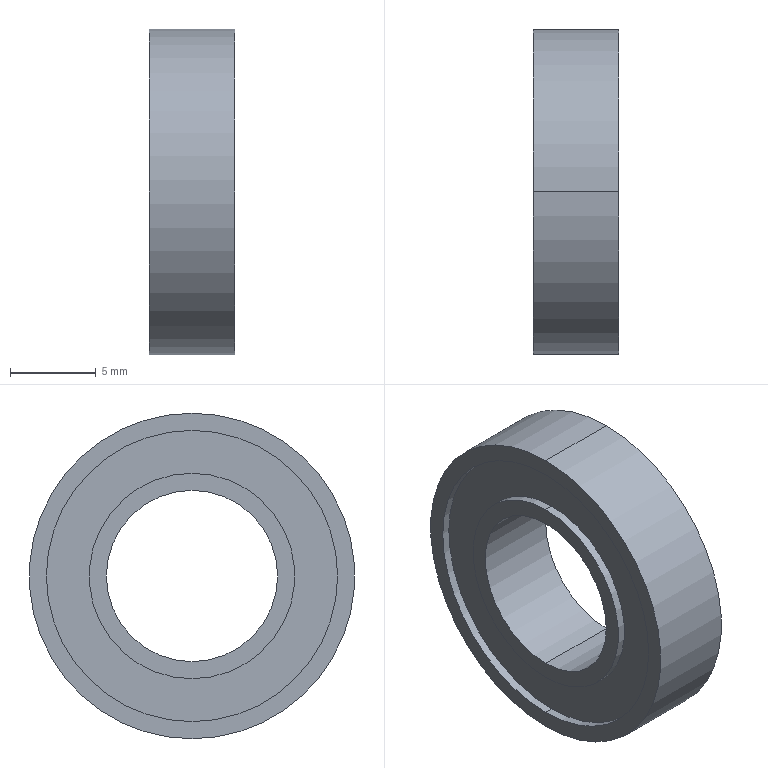Part | STEP file | Guide wheel mechanism revised.sldasm-Part-353 | 1 solid | 18 faces | box 5 x 19 x 19 mm | volume 911.062 mm3 | cylinder 12 | plane 6 | commonest cylinder face diameters 12 x4 17 x4 10 x2 19 x2
STEP:
#1=CARTESIAN_POINT('',(5.,0.,6.));
#2=VERTEX_POINT('',#1);
#3=CARTESIAN_POINT('',(5.,0.,-6.));
#4=VERTEX_POINT('',#3);
#5=CARTESIAN_POINT('',(5.,0.,0.));
#6=DIRECTION('',(-1.,0.,0.));
#7=DIRECTION('',(0.,0.,1.));
#8=AXIS2_PLACEMENT_3D('',#5,#6,#7);
#9=CIRCLE('',#8,6.);
#10=EDGE_CURVE('',#2,#4,#9,.T.);
#11=ORIENTED_EDGE('',*,*,#10,.T.);
#12=CARTESIAN_POINT('',(4.5,0.,-6.));
#13=VERTEX_POINT('',#12);
#14=CARTESIAN_POINT('',(0.,0.,-6.));
#15=DIRECTION('',(-1.,0.,0.));
#16=VECTOR('',#15,1000.);
#17=LINE('',#14,#16);
#18=EDGE_CURVE('',#4,#13,#17,.T.);
#19=ORIENTED_EDGE('',*,*,#18,.T.);
#20=CARTESIAN_POINT('',(4.5,0.,6.));
#21=VERTEX_POINT('',#20);
#22=CARTESIAN_POINT('',(4.5,0.,0.));
#23=DIRECTION('',(-1.,0.,0.));
#24=DIRECTION('',(0.,0.,1.));
#25=AXIS2_PLACEMENT_3D('',#22,#23,#24);
#26=CIRCLE('',#25,6.);
#27=EDGE_CURVE('',#21,#13,#26,.T.);
#28=ORIENTED_EDGE('',*,*,#27,.F.);
#29=CARTESIAN_POINT('',(0.,0.,6.));
#30=DIRECTION('',(-1.,0.,0.));
#31=VECTOR('',#30,1000.);
#32=LINE('',#29,#31);
#33=EDGE_CURVE('',#2,#21,#32,.T.);
#34=ORIENTED_EDGE('',*,*,#33,.F.);
#35=EDGE_LOOP('',(#11,#19,#28,#34));
#36=FACE_OUTER_BOUND('',#35,.T.);
#37=CARTESIAN_POINT('',(0.,0.,0.));
#38=DIRECTION('',(-1.,0.,0.));
#39=DIRECTION('',(0.,0.,1.));
#40=AXIS2_PLACEMENT_3D('',#37,#38,#39);
#41=CYLINDRICAL_SURFACE('',#40,6.);
#42=ADVANCED_FACE('',(#36),#41,.T.);
#43=CARTESIAN_POINT('',(5.,0.,-8.5));
#44=VERTEX_POINT('',#43);
#45=CARTESIAN_POINT('',(5.,0.,8.5));
#46=VERTEX_POINT('',#45);
#47=CARTESIAN_POINT('',(5.,0.,0.));
#48=DIRECTION('',(-1.,0.,0.));
#49=DIRECTION('',(0.,0.,1.));
#50=AXIS2_PLACEMENT_3D('',#47,#48,#49);
#51=CIRCLE('',#50,8.5);
#52=EDGE_CURVE('',#44,#46,#51,.T.);
#53=ORIENTED_EDGE('',*,*,#52,.F.);
#54=CARTESIAN_POINT('',(4.5,0.,-8.5));
#55=VERTEX_POINT('',#54);
#56=CARTESIAN_POINT('',(0.,0.,-8.5));
#57=DIRECTION('',(-1.,0.,0.));
#58=VECTOR('',#57,1000.);
#59=LINE('',#56,#58);
#60=EDGE_CURVE('',#44,#55,#59,.T.);
#61=ORIENTED_EDGE('',*,*,#60,.T.);
#62=CARTESIAN_POINT('',(4.5,0.,8.5));
#63=VERTEX_POINT('',#62);
#64=CARTESIAN_POINT('',(4.5,0.,0.));
#65=DIRECTION('',(-1.,0.,0.));
#66=DIRECTION('',(0.,0.,1.));
#67=AXIS2_PLACEMENT_3D('',#64,#65,#66);
#68=CIRCLE('',#67,8.5);
#69=EDGE_CURVE('',#55,#63,#68,.T.);
#70=ORIENTED_EDGE('',*,*,#69,.T.);
#71=CARTESIAN_POINT('',(0.,0.,8.5));
#72=DIRECTION('',(-1.,0.,0.));
#73=VECTOR('',#72,1000.);
#74=LINE('',#71,#73);
#75=EDGE_CURVE('',#46,#63,#74,.T.);
#76=ORIENTED_EDGE('',*,*,#75,.F.);
#77=EDGE_LOOP('',(#53,#61,#70,#76));
#78=FACE_OUTER_BOUND('',#77,.T.);
#79=CARTESIAN_POINT('',(0.,0.,0.));
#80=DIRECTION('',(-1.,0.,0.));
#81=DIRECTION('',(0.,0.,1.));
#82=AXIS2_PLACEMENT_3D('',#79,#80,#81);
#83=CYLINDRICAL_SURFACE('',#82,8.5);
#84=ADVANCED_FACE('',(#78),#83,.F.);
#85=CARTESIAN_POINT('',(5.,0.,9.5));
#86=VERTEX_POINT('',#85);
#87=CARTESIAN_POINT('',(5.,0.,-9.5));
#88=VERTEX_POINT('',#87);
#89=CARTESIAN_POINT('',(5.,0.,0.));
#90=DIRECTION('',(-1.,0.,0.));
#91=DIRECTION('',(0.,0.,1.));
#92=AXIS2_PLACEMENT_3D('',#89,#90,#91);
#93=CIRCLE('',#92,9.5);
#94=EDGE_CURVE('',#86,#88,#93,.T.);
#95=ORIENTED_EDGE('',*,*,#94,.T.);
#96=CARTESIAN_POINT('',(0.,0.,-9.5));
#97=VERTEX_POINT('',#96);
#98=CARTESIAN_POINT('',(0.,0.,-9.5));
#99=DIRECTION('',(-1.,0.,0.));
#100=VECTOR('',#99,1000.);
#101=LINE('',#98,#100);
#102=EDGE_CURVE('',#88,#97,#101,.T.);
#103=ORIENTED_EDGE('',*,*,#102,.T.);
#104=CARTESIAN_POINT('',(0.,0.,9.5));
#105=VERTEX_POINT('',#104);
#106=CARTESIAN_POINT('',(0.,0.,0.));
#107=DIRECTION('',(-1.,0.,0.));
#108=DIRECTION('',(0.,0.,1.));
#109=AXIS2_PLACEMENT_3D('',#106,#107,#108);
#110=CIRCLE('',#109,9.5);
#111=EDGE_CURVE('',#105,#97,#110,.T.);
#112=ORIENTED_EDGE('',*,*,#111,.F.);
#113=CARTESIAN_POINT('',(0.,0.,9.5));
#114=DIRECTION('',(-1.,0.,0.));
#115=VECTOR('',#114,1000.);
#116=LINE('',#113,#115);
#117=EDGE_CURVE('',#86,#105,#116,.T.);
#118=ORIENTED_EDGE('',*,*,#117,.F.);
#119=EDGE_LOOP('',(#95,#103,#112,#118));
#120=FACE_OUTER_BOUND('',#119,.T.);
#121=CARTESIAN_POINT('',(0.,0.,0.));
#122=DIRECTION('',(-1.,0.,0.));
#123=DIRECTION('',(0.,0.,1.));
#124=AXIS2_PLACEMENT_3D('',#121,#122,#123);
#125=CYLINDRICAL_SURFACE('',#124,9.5);
#126=ADVANCED_FACE('',(#120),#125,.T.);
#127=CARTESIAN_POINT('',(0.5,0.,-8.5));
#128=VERTEX_POINT('',#127);
#129=CARTESIAN_POINT('',(0.5,0.,8.5));
#130=VERTEX_POINT('',#129);
#131=CARTESIAN_POINT('',(0.5,0.,0.));
#132=DIRECTION('',(-1.,0.,0.));
#133=DIRECTION('',(0.,0.,1.));
#134=AXIS2_PLACEMENT_3D('',#131,#132,#133);
#135=CIRCLE('',#134,8.5);
#136=EDGE_CURVE('',#128,#130,#135,.T.);
#137=ORIENTED_EDGE('',*,*,#136,.F.);
#138=CARTESIAN_POINT('',(0.,0.,-8.5));
#139=VERTEX_POINT('',#138);
#140=CARTESIAN_POINT('',(0.,0.,-8.5));
#141=DIRECTION('',(-1.,0.,0.));
#142=VECTOR('',#141,1000.);
#143=LINE('',#140,#142);
#144=EDGE_CURVE('',#128,#139,#143,.T.);
#145=ORIENTED_EDGE('',*,*,#144,.T.);
#146=CARTESIAN_POINT('',(0.,0.,8.5));
#147=VERTEX_POINT('',#146);
#148=CARTESIAN_POINT('',(0.,0.,0.));
#149=DIRECTION('',(-1.,0.,0.));
#150=DIRECTION('',(0.,0.,1.));
#151=AXIS2_PLACEMENT_3D('',#148,#149,#150);
#152=CIRCLE('',#151,8.5);
#153=EDGE_CURVE('',#139,#147,#152,.T.);
#154=ORIENTED_EDGE('',*,*,#153,.T.);
#155=CARTESIAN_POINT('',(0.,0.,8.5));
#156=DIRECTION('',(-1.,0.,0.));
#157=VECTOR('',#156,1000.);
#158=LINE('',#155,#157);
#159=EDGE_CURVE('',#130,#147,#158,.T.);
#160=ORIENTED_EDGE('',*,*,#159,.F.);
#161=EDGE_LOOP('',(#137,#145,#154,#160));
#162=FACE_OUTER_BOUND('',#161,.T.);
#163=CARTESIAN_POINT('',(0.,0.,0.));
#164=DIRECTION('',(-1.,0.,0.));
#165=DIRECTION('',(0.,0.,1.));
#166=AXIS2_PLACEMENT_3D('',#163,#164,#165);
#167=CYLINDRICAL_SURFACE('',#166,8.5);
#168=ADVANCED_FACE('',(#162),#167,.F.);
#169=CARTESIAN_POINT('',(0.5,0.,6.));
#170=VERTEX_POINT('',#169);
#171=CARTESIAN_POINT('',(0.5,0.,-6.));
#172=VERTEX_POINT('',#171);
#173=CARTESIAN_POINT('',(0.5,0.,0.));
#174=DIRECTION('',(-1.,0.,0.));
#175=DIRECTION('',(0.,0.,1.));
#176=AXIS2_PLACEMENT_3D('',#173,#174,#175);
#177=CIRCLE('',#176,6.);
#178=EDGE_CURVE('',#170,#172,#177,.T.);
#179=ORIENTED_EDGE('',*,*,#178,.T.);
#180=CARTESIAN_POINT('',(0.,0.,-6.));
#181=VERTEX_POINT('',#180);
#182=CARTESIAN_POINT('',(0.,0.,-6.));
#183=DIRECTION('',(-1.,0.,0.));
#184=VECTOR('',#183,1000.);
#185=LINE('',#182,#184);
#186=EDGE_CURVE('',#172,#181,#185,.T.);
#187=ORIENTED_EDGE('',*,*,#186,.T.);
#188=CARTESIAN_POINT('',(0.,0.,6.));
#189=VERTEX_POINT('',#188);
#190=CARTESIAN_POINT('',(0.,0.,0.));
#191=DIRECTION('',(-1.,0.,0.));
#192=DIRECTION('',(0.,0.,1.));
#193=AXIS2_PLACEMENT_3D('',#190,#191,#192);
#194=CIRCLE('',#193,6.);
#195=EDGE_CURVE('',#189,#181,#194,.T.);
#196=ORIENTED_EDGE('',*,*,#195,.F.);
#197=CARTESIAN_POINT('',(0.,0.,6.));
#198=DIRECTION('',(-1.,0.,0.));
#199=VECTOR('',#198,1000.);
#200=LINE('',#197,#199);
#201=EDGE_CURVE('',#170,#189,#200,.T.);
#202=ORIENTED_EDGE('',*,*,#201,.F.);
#203=EDGE_LOOP('',(#179,#187,#196,#202));
#204=FACE_OUTER_BOUND('',#203,.T.);
#205=CARTESIAN_POINT('',(0.,0.,0.));
#206=DIRECTION('',(-1.,0.,0.));
#207=DIRECTION('',(0.,0.,1.));
#208=AXIS2_PLACEMENT_3D('',#205,#206,#207);
#209=CYLINDRICAL_SURFACE('',#208,6.);
#210=ADVANCED_FACE('',(#204),#209,.T.);
#211=CARTESIAN_POINT('',(5.,0.,-5.));
#212=VERTEX_POINT('',#211);
#213=CARTESIAN_POINT('',(5.,0.,5.));
#214=VERTEX_POINT('',#213);
#215=CARTESIAN_POINT('',(5.,0.,0.));
#216=DIRECTION('',(-1.,0.,0.));
#217=DIRECTION('',(0.,0.,1.));
#218=AXIS2_PLACEMENT_3D('',#215,#216,#217);
#219=CIRCLE('',#218,5.);
#220=EDGE_CURVE('',#212,#214,#219,.T.);
#221=ORIENTED_EDGE('',*,*,#220,.F.);
#222=CARTESIAN_POINT('',(0.,0.,-5.));
#223=VERTEX_POINT('',#222);
#224=CARTESIAN_POINT('',(0.,0.,-5.));
#225=DIRECTION('',(-1.,0.,0.));
#226=VECTOR('',#225,1000.);
#227=LINE('',#224,#226);
#228=EDGE_CURVE('',#212,#223,#227,.T.);
#229=ORIENTED_EDGE('',*,*,#228,.T.);
#230=CARTESIAN_POINT('',(0.,0.,5.));
#231=VERTEX_POINT('',#230);
#232=CARTESIAN_POINT('',(0.,0.,0.));
#233=DIRECTION('',(-1.,0.,0.));
#234=DIRECTION('',(0.,0.,1.));
#235=AXIS2_PLACEMENT_3D('',#232,#233,#234);
#236=CIRCLE('',#235,5.);
#237=EDGE_CURVE('',#223,#231,#236,.T.);
#238=ORIENTED_EDGE('',*,*,#237,.T.);
#239=CARTESIAN_POINT('',(0.,0.,5.));
#240=DIRECTION('',(-1.,0.,0.));
#241=VECTOR('',#240,1000.);
#242=LINE('',#239,#241);
#243=EDGE_CURVE('',#214,#231,#242,.T.);
#244=ORIENTED_EDGE('',*,*,#243,.F.);
#245=EDGE_LOOP('',(#221,#229,#238,#244));
#246=FACE_OUTER_BOUND('',#245,.T.);
#247=CARTESIAN_POINT('',(0.,0.,0.));
#248=DIRECTION('',(-1.,0.,0.));
#249=DIRECTION('',(0.,0.,1.));
#250=AXIS2_PLACEMENT_3D('',#247,#248,#249);
#251=CYLINDRICAL_SURFACE('',#250,5.);
#252=ADVANCED_FACE('',(#246),#251,.F.);
#253=ORIENTED_EDGE('',*,*,#228,.F.);
#254=CARTESIAN_POINT('',(5.,0.,0.));
#255=DIRECTION('',(-1.,0.,0.));
#256=DIRECTION('',(0.,0.,1.));
#257=AXIS2_PLACEMENT_3D('',#254,#255,#256);
#258=CIRCLE('',#257,5.);
#259=EDGE_CURVE('',#214,#212,#258,.T.);
#260=ORIENTED_EDGE('',*,*,#259,.F.);
#261=ORIENTED_EDGE('',*,*,#243,.T.);
#262=CARTESIAN_POINT('',(0.,0.,0.));
#263=DIRECTION('',(-1.,0.,0.));
#264=DIRECTION('',(0.,0.,1.));
#265=AXIS2_PLACEMENT_3D('',#262,#263,#264);
#266=CIRCLE('',#265,5.);
#267=EDGE_CURVE('',#231,#223,#266,.T.);
#268=ORIENTED_EDGE('',*,*,#267,.T.);
#269=EDGE_LOOP('',(#253,#260,#261,#268));
#270=FACE_OUTER_BOUND('',#269,.T.);
#271=CARTESIAN_POINT('',(0.,0.,0.));
#272=DIRECTION('',(-1.,0.,0.));
#273=DIRECTION('',(0.,0.,1.));
#274=AXIS2_PLACEMENT_3D('',#271,#272,#273);
#275=CYLINDRICAL_SURFACE('',#274,5.);
#276=ADVANCED_FACE('',(#270),#275,.F.);
#277=ORIENTED_EDGE('',*,*,#267,.F.);
#278=ORIENTED_EDGE('',*,*,#237,.F.);
#279=EDGE_LOOP('',(#277,#278));
#280=FACE_BOUND('',#279,.T.);
#281=ORIENTED_EDGE('',*,*,#195,.T.);
#282=CARTESIAN_POINT('',(0.,0.,0.));
#283=DIRECTION('',(-1.,0.,0.));
#284=DIRECTION('',(0.,0.,1.));
#285=AXIS2_PLACEMENT_3D('',#282,#283,#284);
#286=CIRCLE('',#285,6.);
#287=EDGE_CURVE('',#181,#189,#286,.T.);
#288=ORIENTED_EDGE('',*,*,#287,.T.);
#289=EDGE_LOOP('',(#281,#288));
#290=FACE_OUTER_BOUND('',#289,.T.);
#291=CARTESIAN_POINT('',(0.,5.,0.));
#292=DIRECTION('',(1.,0.,0.));
#293=DIRECTION('',(0.,0.,-1.));
#294=AXIS2_PLACEMENT_3D('',#291,#292,#293);
#295=PLANE('',#294);
#296=ADVANCED_FACE('',(#280,#290),#295,.F.);
#297=ORIENTED_EDGE('',*,*,#186,.F.);
#298=CARTESIAN_POINT('',(0.5,0.,0.));
#299=DIRECTION('',(-1.,0.,0.));
#300=DIRECTION('',(0.,0.,1.));
#301=AXIS2_PLACEMENT_3D('',#298,#299,#300);
#302=CIRCLE('',#301,6.);
#303=EDGE_CURVE('',#172,#170,#302,.T.);
#304=ORIENTED_EDGE('',*,*,#303,.T.);
#305=ORIENTED_EDGE('',*,*,#201,.T.);
#306=ORIENTED_EDGE('',*,*,#287,.F.);
#307=EDGE_LOOP('',(#297,#304,#305,#306));
#308=FACE_OUTER_BOUND('',#307,.T.);
#309=CARTESIAN_POINT('',(0.,0.,0.));
#310=DIRECTION('',(-1.,0.,0.));
#311=DIRECTION('',(0.,0.,1.));
#312=AXIS2_PLACEMENT_3D('',#309,#310,#311);
#313=CYLINDRICAL_SURFACE('',#312,6.);
#314=ADVANCED_FACE('',(#308),#313,.T.);
#315=ORIENTED_EDGE('',*,*,#178,.F.);
#316=ORIENTED_EDGE('',*,*,#303,.F.);
#317=EDGE_LOOP('',(#315,#316));
#318=FACE_BOUND('',#317,.T.);
#319=CARTESIAN_POINT('',(0.5,0.,0.));
#320=DIRECTION('',(-1.,0.,0.));
#321=DIRECTION('',(0.,0.,1.));
#322=AXIS2_PLACEMENT_3D('',#319,#320,#321);
#323=CIRCLE('',#322,8.5);
#324=EDGE_CURVE('',#130,#128,#323,.T.);
#325=ORIENTED_EDGE('',*,*,#324,.T.);
#326=ORIENTED_EDGE('',*,*,#136,.T.);
#327=EDGE_LOOP('',(#325,#326));
#328=FACE_OUTER_BOUND('',#327,.T.);
#329=CARTESIAN_POINT('',(0.5,6.,0.));
#330=DIRECTION('',(1.,0.,0.));
#331=DIRECTION('',(0.,0.,-1.));
#332=AXIS2_PLACEMENT_3D('',#329,#330,#331);
#333=PLANE('',#332);
#334=ADVANCED_FACE('',(#318,#328),#333,.F.);
#335=ORIENTED_EDGE('',*,*,#144,.F.);
#336=ORIENTED_EDGE('',*,*,#324,.F.);
#337=ORIENTED_EDGE('',*,*,#159,.T.);
#338=CARTESIAN_POINT('',(0.,0.,0.));
#339=DIRECTION('',(-1.,0.,0.));
#340=DIRECTION('',(0.,0.,1.));
#341=AXIS2_PLACEMENT_3D('',#338,#339,#340);
#342=CIRCLE('',#341,8.5);
#343=EDGE_CURVE('',#147,#139,#342,.T.);
#344=ORIENTED_EDGE('',*,*,#343,.T.);
#345=EDGE_LOOP('',(#335,#336,#337,#344));
#346=FACE_OUTER_BOUND('',#345,.T.);
#347=CARTESIAN_POINT('',(0.,0.,0.));
#348=DIRECTION('',(-1.,0.,0.));
#349=DIRECTION('',(0.,0.,1.));
#350=AXIS2_PLACEMENT_3D('',#347,#348,#349);
#351=CYLINDRICAL_SURFACE('',#350,8.5);
#352=ADVANCED_FACE('',(#346),#351,.F.);
#353=ORIENTED_EDGE('',*,*,#343,.F.);
#354=ORIENTED_EDGE('',*,*,#153,.F.);
#355=EDGE_LOOP('',(#353,#354));
#356=FACE_BOUND('',#355,.T.);
#357=ORIENTED_EDGE('',*,*,#111,.T.);
#358=CARTESIAN_POINT('',(0.,0.,0.));
#359=DIRECTION('',(-1.,0.,0.));
#360=DIRECTION('',(0.,0.,1.));
#361=AXIS2_PLACEMENT_3D('',#358,#359,#360);
#362=CIRCLE('',#361,9.5);
#363=EDGE_CURVE('',#97,#105,#362,.T.);
#364=ORIENTED_EDGE('',*,*,#363,.T.);
#365=EDGE_LOOP('',(#357,#364));
#366=FACE_OUTER_BOUND('',#365,.T.);
#367=CARTESIAN_POINT('',(0.,8.5,0.));
#368=DIRECTION('',(1.,0.,0.));
#369=DIRECTION('',(0.,0.,-1.));
#370=AXIS2_PLACEMENT_3D('',#367,#368,#369);
#371=PLANE('',#370);
#372=ADVANCED_FACE('',(#356,#366),#371,.F.);
#373=ORIENTED_EDGE('',*,*,#102,.F.);
#374=CARTESIAN_POINT('',(5.,0.,0.));
#375=DIRECTION('',(-1.,0.,0.));
#376=DIRECTION('',(0.,0.,1.));
#377=AXIS2_PLACEMENT_3D('',#374,#375,#376);
#378=CIRCLE('',#377,9.5);
#379=EDGE_CURVE('',#88,#86,#378,.T.);
#380=ORIENTED_EDGE('',*,*,#379,.T.);
#381=ORIENTED_EDGE('',*,*,#117,.T.);
#382=ORIENTED_EDGE('',*,*,#363,.F.);
#383=EDGE_LOOP('',(#373,#380,#381,#382));
#384=FACE_OUTER_BOUND('',#383,.T.);
#385=CARTESIAN_POINT('',(0.,0.,0.));
#386=DIRECTION('',(-1.,0.,0.));
#387=DIRECTION('',(0.,0.,1.));
#388=AXIS2_PLACEMENT_3D('',#385,#386,#387);
#389=CYLINDRICAL_SURFACE('',#388,9.5);
#390=ADVANCED_FACE('',(#384),#389,.T.);
#391=ORIENTED_EDGE('',*,*,#94,.F.);
#392=ORIENTED_EDGE('',*,*,#379,.F.);
#393=EDGE_LOOP('',(#391,#392));
#394=FACE_OUTER_BOUND('',#393,.T.);
#395=CARTESIAN_POINT('',(5.,0.,0.));
#396=DIRECTION('',(-1.,0.,0.));
#397=DIRECTION('',(0.,0.,1.));
#398=AXIS2_PLACEMENT_3D('',#395,#396,#397);
#399=CIRCLE('',#398,8.5);
#400=EDGE_CURVE('',#46,#44,#399,.T.);
#401=ORIENTED_EDGE('',*,*,#400,.T.);
#402=ORIENTED_EDGE('',*,*,#52,.T.);
#403=EDGE_LOOP('',(#401,#402));
#404=FACE_BOUND('',#403,.T.);
#405=CARTESIAN_POINT('',(5.,9.5,0.));
#406=DIRECTION('',(-1.,0.,0.));
#407=DIRECTION('',(0.,0.,1.));
#408=AXIS2_PLACEMENT_3D('',#405,#406,#407);
#409=PLANE('',#408);
#410=ADVANCED_FACE('',(#394,#404),#409,.F.);
#411=ORIENTED_EDGE('',*,*,#60,.F.);
#412=ORIENTED_EDGE('',*,*,#400,.F.);
#413=ORIENTED_EDGE('',*,*,#75,.T.);
#414=CARTESIAN_POINT('',(4.5,0.,0.));
#415=DIRECTION('',(-1.,0.,0.));
#416=DIRECTION('',(0.,0.,1.));
#417=AXIS2_PLACEMENT_3D('',#414,#415,#416);
#418=CIRCLE('',#417,8.5);
#419=EDGE_CURVE('',#63,#55,#418,.T.);
#420=ORIENTED_EDGE('',*,*,#419,.T.);
#421=EDGE_LOOP('',(#411,#412,#413,#420));
#422=FACE_OUTER_BOUND('',#421,.T.);
#423=CARTESIAN_POINT('',(0.,0.,0.));
#424=DIRECTION('',(-1.,0.,0.));
#425=DIRECTION('',(0.,0.,1.));
#426=AXIS2_PLACEMENT_3D('',#423,#424,#425);
#427=CYLINDRICAL_SURFACE('',#426,8.5);
#428=ADVANCED_FACE('',(#422),#427,.F.);
#429=ORIENTED_EDGE('',*,*,#419,.F.);
#430=ORIENTED_EDGE('',*,*,#69,.F.);
#431=EDGE_LOOP('',(#429,#430));
#432=FACE_OUTER_BOUND('',#431,.T.);
#433=ORIENTED_EDGE('',*,*,#27,.T.);
#434=CARTESIAN_POINT('',(4.5,0.,0.));
#435=DIRECTION('',(-1.,0.,0.));
#436=DIRECTION('',(0.,0.,1.));
#437=AXIS2_PLACEMENT_3D('',#434,#435,#436);
#438=CIRCLE('',#437,6.);
#439=EDGE_CURVE('',#13,#21,#438,.T.);
#440=ORIENTED_EDGE('',*,*,#439,.T.);
#441=EDGE_LOOP('',(#433,#440));
#442=FACE_BOUND('',#441,.T.);
#443=CARTESIAN_POINT('',(4.5,8.5,0.));
#444=DIRECTION('',(-1.,0.,0.));
#445=DIRECTION('',(0.,0.,1.));
#446=AXIS2_PLACEMENT_3D('',#443,#444,#445);
#447=PLANE('',#446);
#448=ADVANCED_FACE('',(#432,#442),#447,.F.);
#449=ORIENTED_EDGE('',*,*,#18,.F.);
#450=CARTESIAN_POINT('',(5.,0.,0.));
#451=DIRECTION('',(-1.,0.,0.));
#452=DIRECTION('',(0.,0.,1.));
#453=AXIS2_PLACEMENT_3D('',#450,#451,#452);
#454=CIRCLE('',#453,6.);
#455=EDGE_CURVE('',#4,#2,#454,.T.);
#456=ORIENTED_EDGE('',*,*,#455,.T.);
#457=ORIENTED_EDGE('',*,*,#33,.T.);
#458=ORIENTED_EDGE('',*,*,#439,.F.);
#459=EDGE_LOOP('',(#449,#456,#457,#458));
#460=FACE_OUTER_BOUND('',#459,.T.);
#461=CARTESIAN_POINT('',(0.,0.,0.));
#462=DIRECTION('',(-1.,0.,0.));
#463=DIRECTION('',(0.,0.,1.));
#464=AXIS2_PLACEMENT_3D('',#461,#462,#463);
#465=CYLINDRICAL_SURFACE('',#464,6.);
#466=ADVANCED_FACE('',(#460),#465,.T.);
#467=ORIENTED_EDGE('',*,*,#10,.F.);
#468=ORIENTED_EDGE('',*,*,#455,.F.);
#469=EDGE_LOOP('',(#467,#468));
#470=FACE_OUTER_BOUND('',#469,.T.);
#471=ORIENTED_EDGE('',*,*,#259,.T.);
#472=ORIENTED_EDGE('',*,*,#220,.T.);
#473=EDGE_LOOP('',(#471,#472));
#474=FACE_BOUND('',#473,.T.);
#475=CARTESIAN_POINT('',(5.,6.,0.));
#476=DIRECTION('',(-1.,0.,0.));
#477=DIRECTION('',(0.,0.,1.));
#478=AXIS2_PLACEMENT_3D('',#475,#476,#477);
#479=PLANE('',#478);
#480=ADVANCED_FACE('',(#470,#474),#479,.F.);
#481=CLOSED_SHELL('',(#42,#84,#126,#168,#210,#252,#276,#296,#314,#334,#352,#372,#390,#410,#428,#448,#466,#480));
#482=MANIFOLD_SOLID_BREP('',#481);
#483=CARTESIAN_POINT('',(0.,0.,0.));
#484=DIRECTION('',(0.,0.,1.));
#485=DIRECTION('',(1.,0.,0.));
#486=AXIS2_PLACEMENT_3D('',#483,#484,#485);
#487=(LENGTH_UNIT()NAMED_UNIT(*)SI_UNIT(.MILLI.,.METRE.));
#488=UNCERTAINTY_MEASURE_WITH_UNIT(LENGTH_MEASURE(0.00001),#487,'','');
#489=(NAMED_UNIT(*)PLANE_ANGLE_UNIT()SI_UNIT($,.RADIAN.));
#490=(NAMED_UNIT(*)SI_UNIT($,.STERADIAN.)SOLID_ANGLE_UNIT());
#491=(GEOMETRIC_REPRESENTATION_CONTEXT(3)GLOBAL_UNCERTAINTY_ASSIGNED_CONTEXT((#488))GLOBAL_UNIT_ASSIGNED_CONTEXT((#487,#489,#490))REPRESENTATION_CONTEXT('',''));
#492=ADVANCED_BREP_SHAPE_REPRESENTATION('',(#482,#486),#491);